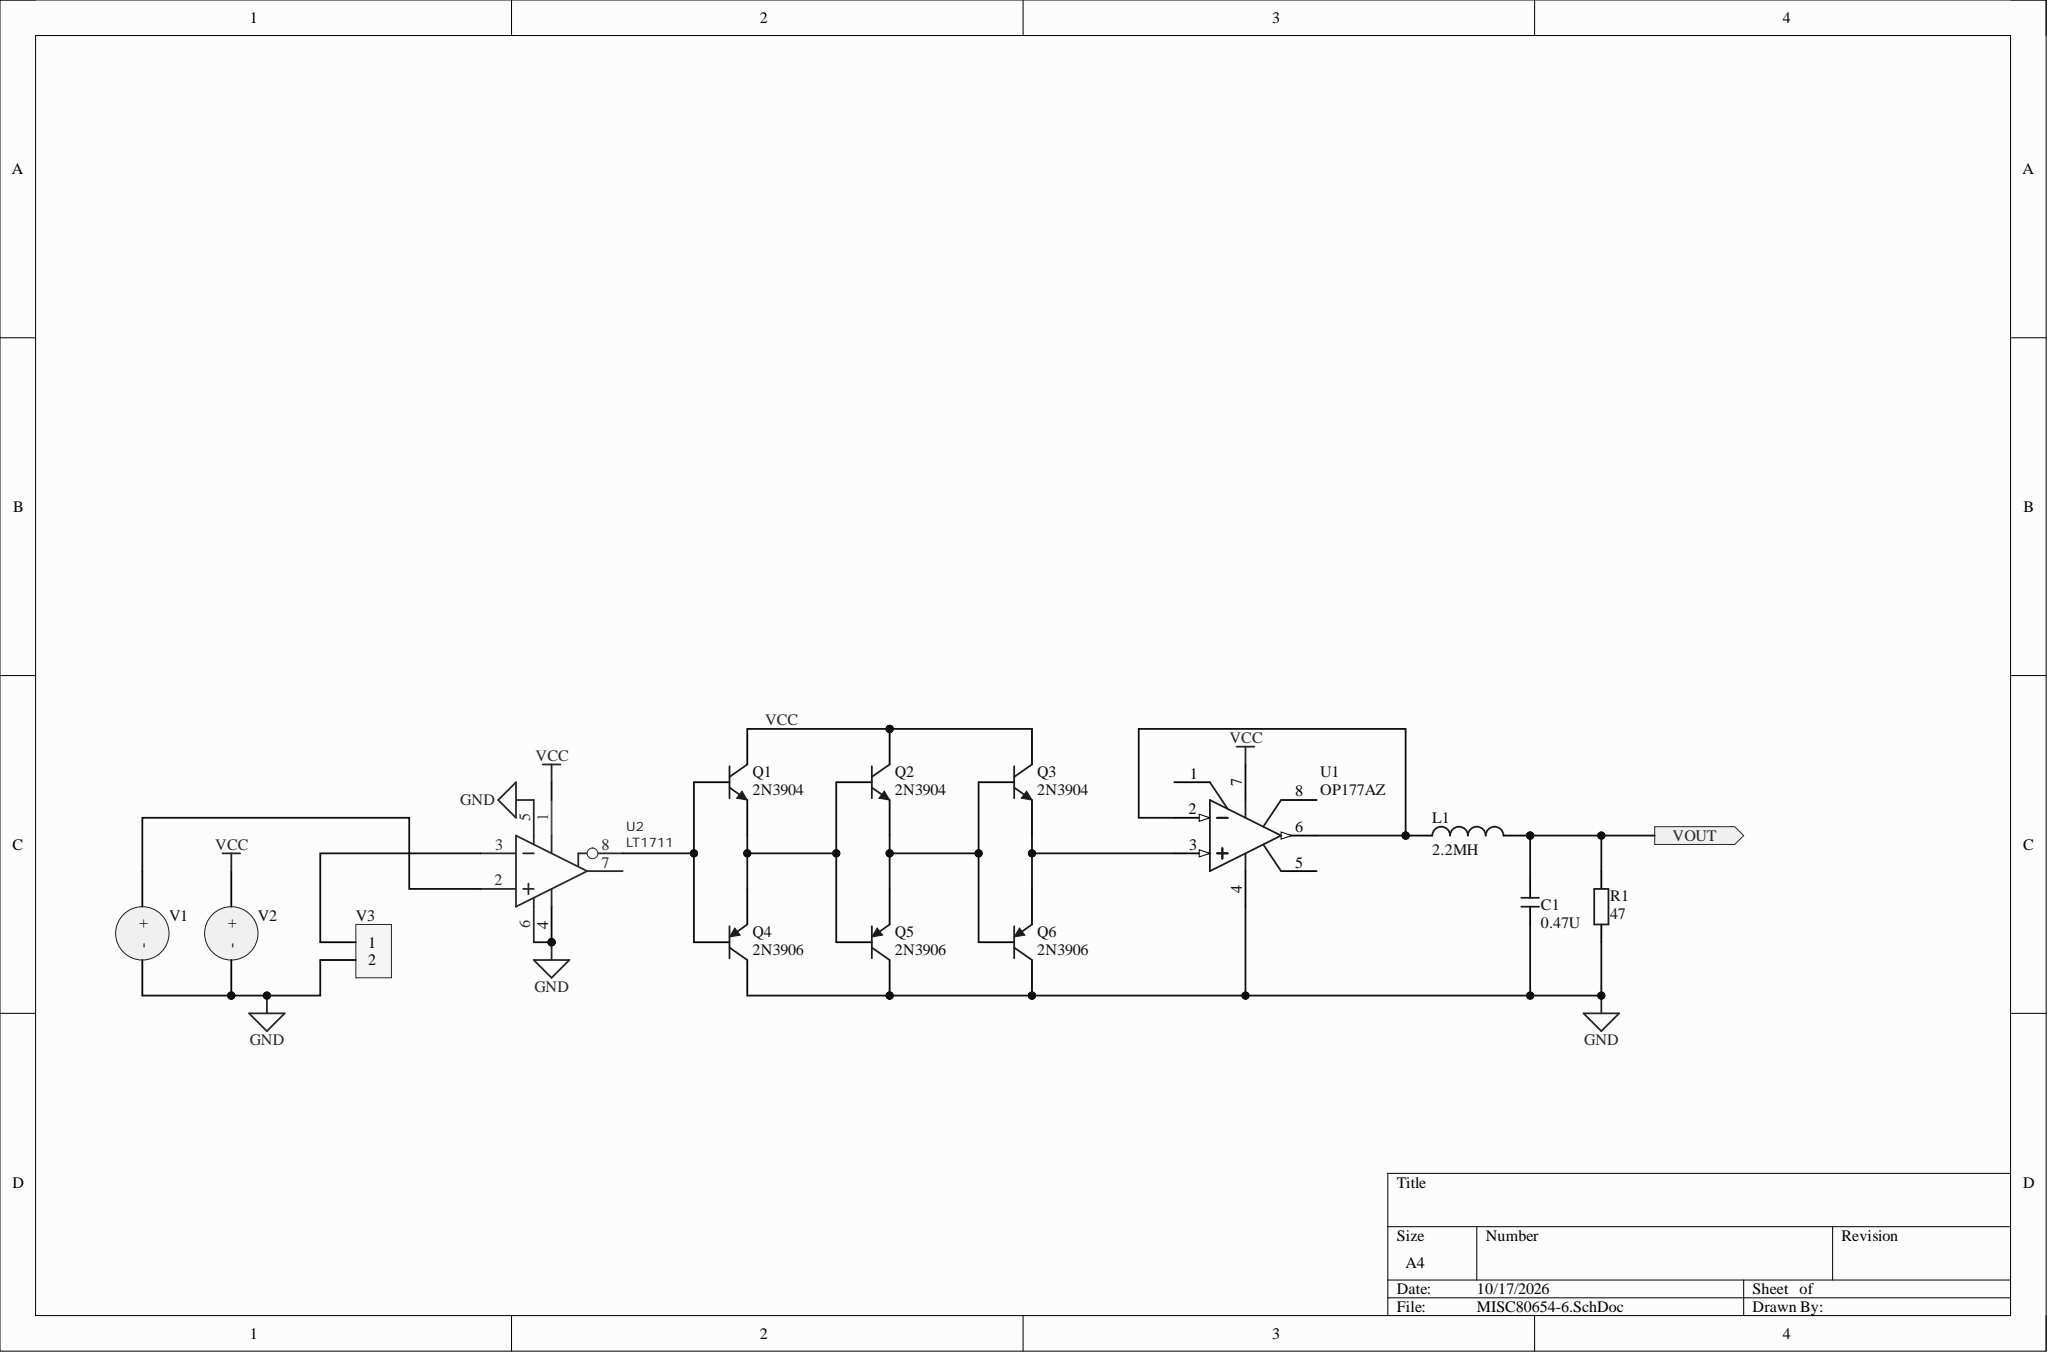Circuit board | Altium Designer | 14 parts | 10 nets
Bill of materials:
Comment,Description,Designator,Footprint,LibRef,Quantity
"0.47U","Ceramic disc capacitor","C1","CC 1.8*3.6","CC","1"
"2.2MH","Color-band inductor","L1","AL0307","L-AL","1"
"2N3904","NPN General Purpose Amplifier","Q1, Q2, Q3","TO-92A","2N3904","3"
"2N3906","PNP General Purpose Amplifier","Q4, Q5, Q6","TO-92A","2N3906","3"
"47","Color-band resistor","R1","RS 1/4W","R-S","1"
"OP177AZ","Ultraprecision Operational Amplifier","U1","Q-8","OP177AZ","1"
"LT1711","","U2","SOP8","LT1711CMS8#PBF","1"
"Current source","","V1, V2","Fe-HDR1X2/2.54-S","电流源","2"
"Female HDR1X2","","V3","Fe-HDR1X2/2.54-S","Female HDR1X2","1"
Netlist (Protel format):
[
C1
CC 1.8*3.6
0.47U



]
[
L1
AL0307
2.2MH



]
[
Q1
TO-92A
2N3904



]
[
Q2
TO-92A
2N3904



]
[
Q3
TO-92A
2N3904



]
[
Q4
TO-92A
2N3906



]
[
Q5
TO-92A
2N3906



]
[
Q6
TO-92A
2N3906



]
[
R1
RS 1/4W
47



]
[
U1
Q-8
OP177AZ



]
[
U2
SOP8
LT1711



]
[
V1
Fe-HDR1X2/2.54-S
Current source



]
[
V2
Fe-HDR1X2/2.54-S
Current source



]
[
V3
Fe-HDR1X2/2.54-S
Female HDR1X2



]
(
VCC
Q1-3
Q2-3
Q3-3
U1-7
U2-1
V2-1
)
(
NetU2_3
U2-3
V3-1
)
(
NetU2_2
U2-2
V1-1
)
(
NetQ3_1
Q3-1
Q6-1
U1-3
)
(
NetQ2_1
Q2-1
Q3-2
Q5-1
Q6-2
)
(
NetQ1_2
Q1-2
Q4-2
U2-8
)
(
NetQ1_1
Q1-1
Q2-2
Q4-1
Q5-2
)
(
NetL1_1
L1-1
U1-2
U1-6
)
(
NetC1_1
C1-1
L1-2
R1-2
)
(
GND
C1-2
Q4-3
Q5-3
Q6-3
R1-1
U1-4
U2-4
U2-5
U2-6
V1-2
V2-2
V3-2
)